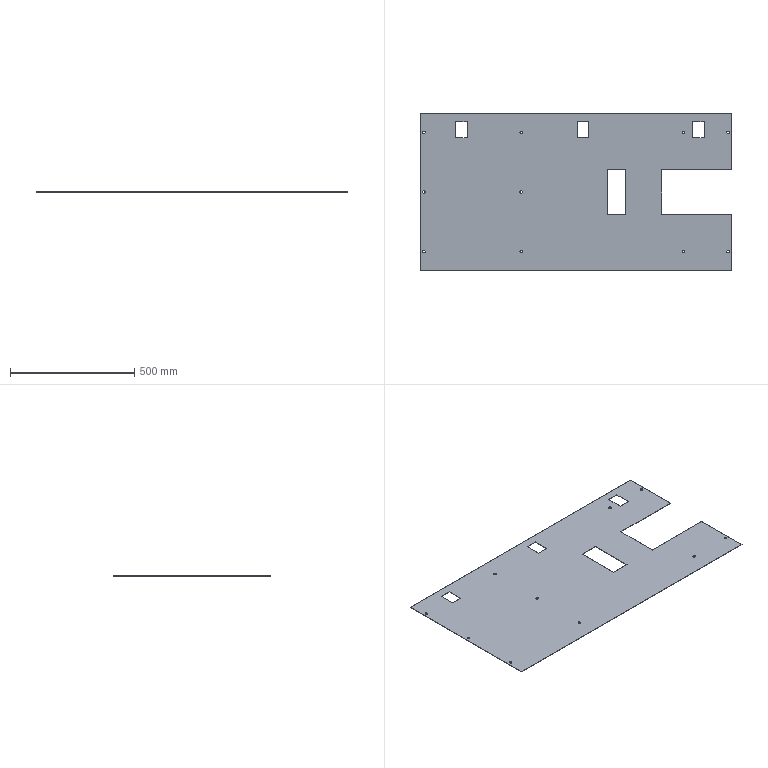Part | STEP file | 1 solid | 46 faces | box 1255 x 636 x 1.5 mm | volume 1086247 mm3 | plane 26 | cylinder 20 | commonest cylinder face diameters 10 x20